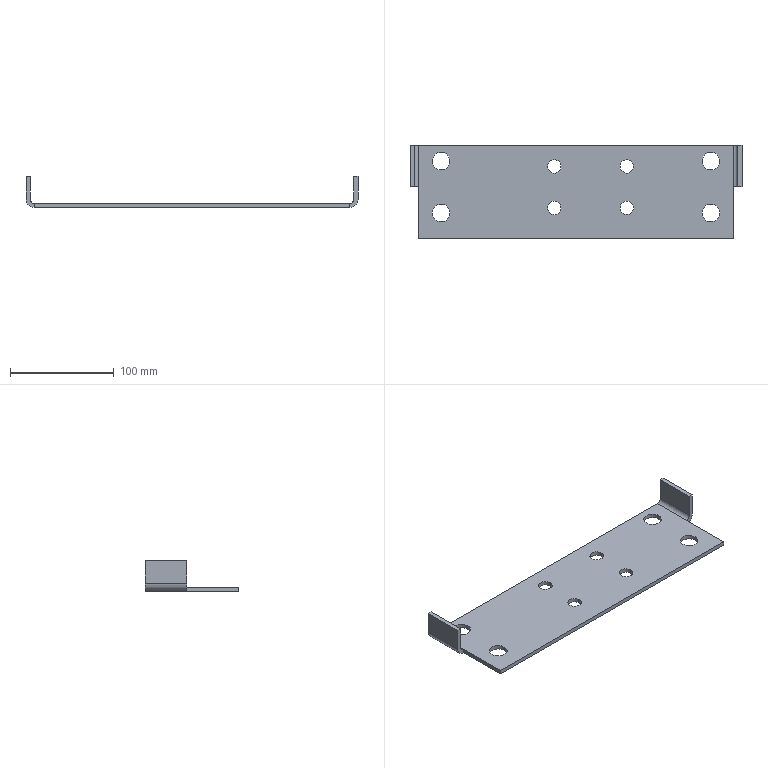Part | SolidWorks | features ICE 3, FlatPattern 1, SMBaseFlange 1, SheetMetal 1 | 1 solid | 38 faces | box 320 x 90.5 x 30 mm | volume 114349 mm3 | cylinder 20 | plane 18 | commonest cylinder face diameters 13 x8 17 x8 8 x2 16 x2
STEP:
#1=CARTESIAN_POINT('',(55.5,-15.25,4.));
#2=VERTEX_POINT('',#1);
#3=CARTESIAN_POINT('',(42.5,-15.25,4.));
#4=VERTEX_POINT('',#3);
#5=CARTESIAN_POINT('',(49.,-15.25,4.));
#6=DIRECTION('',(0.,0.,-1.));
#7=DIRECTION('',(-1.,0.,0.));
#8=AXIS2_PLACEMENT_3D('',#5,#6,#7);
#9=CIRCLE('',#8,6.5);
#10=EDGE_CURVE('',#2,#4,#9,.T.);
#11=ORIENTED_EDGE('',*,*,#10,.F.);
#12=CARTESIAN_POINT('',(55.5,-15.25,0.));
#13=VERTEX_POINT('',#12);
#14=CARTESIAN_POINT('',(55.5,-15.25,10.));
#15=DIRECTION('',(0.,0.,-1.));
#16=VECTOR('',#15,1000.);
#17=LINE('',#14,#16);
#18=EDGE_CURVE('',#2,#13,#17,.T.);
#19=ORIENTED_EDGE('',*,*,#18,.T.);
#20=CARTESIAN_POINT('',(42.5,-15.25,0.));
#21=VERTEX_POINT('',#20);
#22=CARTESIAN_POINT('',(49.,-15.25,0.));
#23=DIRECTION('',(0.,0.,-1.));
#24=DIRECTION('',(-1.,0.,0.));
#25=AXIS2_PLACEMENT_3D('',#22,#23,#24);
#26=CIRCLE('',#25,6.5);
#27=EDGE_CURVE('',#13,#21,#26,.T.);
#28=ORIENTED_EDGE('',*,*,#27,.T.);
#29=CARTESIAN_POINT('',(42.5,-15.25,10.));
#30=DIRECTION('',(0.,0.,-1.));
#31=VECTOR('',#30,1000.);
#32=LINE('',#29,#31);
#33=EDGE_CURVE('',#4,#21,#32,.T.);
#34=ORIENTED_EDGE('',*,*,#33,.F.);
#35=EDGE_LOOP('',(#11,#19,#28,#34));
#36=FACE_OUTER_BOUND('',#35,.T.);
#37=CARTESIAN_POINT('',(49.,-15.25,10.));
#38=DIRECTION('',(0.,0.,-1.));
#39=DIRECTION('',(-1.,0.,0.));
#40=AXIS2_PLACEMENT_3D('',#37,#38,#39);
#41=CYLINDRICAL_SURFACE('',#40,6.5);
#42=ADVANCED_FACE('',(#36),#41,.F.);
#43=CARTESIAN_POINT('',(-14.5,24.75,4.));
#44=VERTEX_POINT('',#43);
#45=CARTESIAN_POINT('',(-27.5,24.75,4.));
#46=VERTEX_POINT('',#45);
#47=CARTESIAN_POINT('',(-21.,24.75,4.));
#48=DIRECTION('',(0.,0.,-1.));
#49=DIRECTION('',(-1.,0.,0.));
#50=AXIS2_PLACEMENT_3D('',#47,#48,#49);
#51=CIRCLE('',#50,6.5);
#52=EDGE_CURVE('',#44,#46,#51,.T.);
#53=ORIENTED_EDGE('',*,*,#52,.F.);
#54=CARTESIAN_POINT('',(-14.5,24.75,0.));
#55=VERTEX_POINT('',#54);
#56=CARTESIAN_POINT('',(-14.5,24.75,10.));
#57=DIRECTION('',(0.,0.,-1.));
#58=VECTOR('',#57,1000.);
#59=LINE('',#56,#58);
#60=EDGE_CURVE('',#44,#55,#59,.T.);
#61=ORIENTED_EDGE('',*,*,#60,.T.);
#62=CARTESIAN_POINT('',(-27.5,24.75,0.));
#63=VERTEX_POINT('',#62);
#64=CARTESIAN_POINT('',(-21.,24.75,0.));
#65=DIRECTION('',(0.,0.,-1.));
#66=DIRECTION('',(-1.,0.,0.));
#67=AXIS2_PLACEMENT_3D('',#64,#65,#66);
#68=CIRCLE('',#67,6.5);
#69=EDGE_CURVE('',#55,#63,#68,.T.);
#70=ORIENTED_EDGE('',*,*,#69,.T.);
#71=CARTESIAN_POINT('',(-27.5,24.75,10.));
#72=DIRECTION('',(0.,0.,-1.));
#73=VECTOR('',#72,1000.);
#74=LINE('',#71,#73);
#75=EDGE_CURVE('',#46,#63,#74,.T.);
#76=ORIENTED_EDGE('',*,*,#75,.F.);
#77=EDGE_LOOP('',(#53,#61,#70,#76));
#78=FACE_OUTER_BOUND('',#77,.T.);
#79=CARTESIAN_POINT('',(-21.,24.75,10.));
#80=DIRECTION('',(0.,0.,-1.));
#81=DIRECTION('',(-1.,0.,0.));
#82=AXIS2_PLACEMENT_3D('',#79,#80,#81);
#83=CYLINDRICAL_SURFACE('',#82,6.5);
#84=ADVANCED_FACE('',(#78),#83,.F.);
#85=CARTESIAN_POINT('',(-14.5,-15.25,4.));
#86=VERTEX_POINT('',#85);
#87=CARTESIAN_POINT('',(-27.5,-15.25,4.));
#88=VERTEX_POINT('',#87);
#89=CARTESIAN_POINT('',(-21.,-15.25,4.));
#90=DIRECTION('',(0.,0.,-1.));
#91=DIRECTION('',(-1.,0.,0.));
#92=AXIS2_PLACEMENT_3D('',#89,#90,#91);
#93=CIRCLE('',#92,6.5);
#94=EDGE_CURVE('',#86,#88,#93,.T.);
#95=ORIENTED_EDGE('',*,*,#94,.F.);
#96=CARTESIAN_POINT('',(-14.5,-15.25,0.));
#97=VERTEX_POINT('',#96);
#98=CARTESIAN_POINT('',(-14.5,-15.25,10.));
#99=DIRECTION('',(0.,0.,-1.));
#100=VECTOR('',#99,1000.);
#101=LINE('',#98,#100);
#102=EDGE_CURVE('',#86,#97,#101,.T.);
#103=ORIENTED_EDGE('',*,*,#102,.T.);
#104=CARTESIAN_POINT('',(-27.5,-15.25,0.));
#105=VERTEX_POINT('',#104);
#106=CARTESIAN_POINT('',(-21.,-15.25,0.));
#107=DIRECTION('',(0.,0.,-1.));
#108=DIRECTION('',(-1.,0.,0.));
#109=AXIS2_PLACEMENT_3D('',#106,#107,#108);
#110=CIRCLE('',#109,6.5);
#111=EDGE_CURVE('',#97,#105,#110,.T.);
#112=ORIENTED_EDGE('',*,*,#111,.T.);
#113=CARTESIAN_POINT('',(-27.5,-15.25,10.));
#114=DIRECTION('',(0.,0.,-1.));
#115=VECTOR('',#114,1000.);
#116=LINE('',#113,#115);
#117=EDGE_CURVE('',#88,#105,#116,.T.);
#118=ORIENTED_EDGE('',*,*,#117,.F.);
#119=EDGE_LOOP('',(#95,#103,#112,#118));
#120=FACE_OUTER_BOUND('',#119,.T.);
#121=CARTESIAN_POINT('',(-21.,-15.25,10.));
#122=DIRECTION('',(0.,0.,-1.));
#123=DIRECTION('',(-1.,0.,0.));
#124=AXIS2_PLACEMENT_3D('',#121,#122,#123);
#125=CYLINDRICAL_SURFACE('',#124,6.5);
#126=ADVANCED_FACE('',(#120),#125,.F.);
#127=CARTESIAN_POINT('',(55.5,24.75,4.));
#128=VERTEX_POINT('',#127);
#129=CARTESIAN_POINT('',(42.5,24.75,4.));
#130=VERTEX_POINT('',#129);
#131=CARTESIAN_POINT('',(49.,24.75,4.));
#132=DIRECTION('',(0.,0.,-1.));
#133=DIRECTION('',(-1.,0.,0.));
#134=AXIS2_PLACEMENT_3D('',#131,#132,#133);
#135=CIRCLE('',#134,6.5);
#136=EDGE_CURVE('',#128,#130,#135,.T.);
#137=ORIENTED_EDGE('',*,*,#136,.F.);
#138=CARTESIAN_POINT('',(55.5,24.75,0.));
#139=VERTEX_POINT('',#138);
#140=CARTESIAN_POINT('',(55.5,24.75,10.));
#141=DIRECTION('',(0.,0.,-1.));
#142=VECTOR('',#141,1000.);
#143=LINE('',#140,#142);
#144=EDGE_CURVE('',#128,#139,#143,.T.);
#145=ORIENTED_EDGE('',*,*,#144,.T.);
#146=CARTESIAN_POINT('',(42.5,24.75,0.));
#147=VERTEX_POINT('',#146);
#148=CARTESIAN_POINT('',(49.,24.75,0.));
#149=DIRECTION('',(0.,0.,-1.));
#150=DIRECTION('',(-1.,0.,0.));
#151=AXIS2_PLACEMENT_3D('',#148,#149,#150);
#152=CIRCLE('',#151,6.5);
#153=EDGE_CURVE('',#139,#147,#152,.T.);
#154=ORIENTED_EDGE('',*,*,#153,.T.);
#155=CARTESIAN_POINT('',(42.5,24.75,10.));
#156=DIRECTION('',(0.,0.,-1.));
#157=VECTOR('',#156,1000.);
#158=LINE('',#155,#157);
#159=EDGE_CURVE('',#130,#147,#158,.T.);
#160=ORIENTED_EDGE('',*,*,#159,.F.);
#161=EDGE_LOOP('',(#137,#145,#154,#160));
#162=FACE_OUTER_BOUND('',#161,.T.);
#163=CARTESIAN_POINT('',(49.,24.75,10.));
#164=DIRECTION('',(0.,0.,-1.));
#165=DIRECTION('',(-1.,0.,0.));
#166=AXIS2_PLACEMENT_3D('',#163,#164,#165);
#167=CYLINDRICAL_SURFACE('',#166,6.5);
#168=ADVANCED_FACE('',(#162),#167,.F.);
#169=CARTESIAN_POINT('',(-121.5,-20.25,4.));
#170=VERTEX_POINT('',#169);
#171=CARTESIAN_POINT('',(-138.5,-20.25,4.));
#172=VERTEX_POINT('',#171);
#173=CARTESIAN_POINT('',(-130.,-20.25,4.));
#174=DIRECTION('',(0.,0.,-1.));
#175=DIRECTION('',(-1.,0.,0.));
#176=AXIS2_PLACEMENT_3D('',#173,#174,#175);
#177=CIRCLE('',#176,8.5);
#178=EDGE_CURVE('',#170,#172,#177,.T.);
#179=ORIENTED_EDGE('',*,*,#178,.F.);
#180=CARTESIAN_POINT('',(-121.5,-20.25,0.));
#181=VERTEX_POINT('',#180);
#182=CARTESIAN_POINT('',(-121.5,-20.25,10.));
#183=DIRECTION('',(0.,0.,-1.));
#184=VECTOR('',#183,1000.);
#185=LINE('',#182,#184);
#186=EDGE_CURVE('',#170,#181,#185,.T.);
#187=ORIENTED_EDGE('',*,*,#186,.T.);
#188=CARTESIAN_POINT('',(-138.5,-20.25,0.));
#189=VERTEX_POINT('',#188);
#190=CARTESIAN_POINT('',(-130.,-20.25,0.));
#191=DIRECTION('',(0.,0.,-1.));
#192=DIRECTION('',(-1.,0.,0.));
#193=AXIS2_PLACEMENT_3D('',#190,#191,#192);
#194=CIRCLE('',#193,8.5);
#195=EDGE_CURVE('',#181,#189,#194,.T.);
#196=ORIENTED_EDGE('',*,*,#195,.T.);
#197=CARTESIAN_POINT('',(-138.5,-20.25,10.));
#198=DIRECTION('',(0.,0.,-1.));
#199=VECTOR('',#198,1000.);
#200=LINE('',#197,#199);
#201=EDGE_CURVE('',#172,#189,#200,.T.);
#202=ORIENTED_EDGE('',*,*,#201,.F.);
#203=EDGE_LOOP('',(#179,#187,#196,#202));
#204=FACE_OUTER_BOUND('',#203,.T.);
#205=CARTESIAN_POINT('',(-130.,-20.25,10.));
#206=DIRECTION('',(0.,0.,-1.));
#207=DIRECTION('',(-1.,0.,0.));
#208=AXIS2_PLACEMENT_3D('',#205,#206,#207);
#209=CYLINDRICAL_SURFACE('',#208,8.5);
#210=ADVANCED_FACE('',(#204),#209,.F.);
#211=CARTESIAN_POINT('',(138.5,-20.25,4.));
#212=VERTEX_POINT('',#211);
#213=CARTESIAN_POINT('',(121.5,-20.25,4.));
#214=VERTEX_POINT('',#213);
#215=CARTESIAN_POINT('',(130.,-20.25,4.));
#216=DIRECTION('',(0.,0.,-1.));
#217=DIRECTION('',(-1.,0.,0.));
#218=AXIS2_PLACEMENT_3D('',#215,#216,#217);
#219=CIRCLE('',#218,8.5);
#220=EDGE_CURVE('',#212,#214,#219,.T.);
#221=ORIENTED_EDGE('',*,*,#220,.F.);
#222=CARTESIAN_POINT('',(138.5,-20.25,0.));
#223=VERTEX_POINT('',#222);
#224=CARTESIAN_POINT('',(138.5,-20.25,10.));
#225=DIRECTION('',(0.,0.,-1.));
#226=VECTOR('',#225,1000.);
#227=LINE('',#224,#226);
#228=EDGE_CURVE('',#212,#223,#227,.T.);
#229=ORIENTED_EDGE('',*,*,#228,.T.);
#230=CARTESIAN_POINT('',(121.5,-20.25,0.));
#231=VERTEX_POINT('',#230);
#232=CARTESIAN_POINT('',(130.,-20.25,0.));
#233=DIRECTION('',(0.,0.,-1.));
#234=DIRECTION('',(-1.,0.,0.));
#235=AXIS2_PLACEMENT_3D('',#232,#233,#234);
#236=CIRCLE('',#235,8.5);
#237=EDGE_CURVE('',#223,#231,#236,.T.);
#238=ORIENTED_EDGE('',*,*,#237,.T.);
#239=CARTESIAN_POINT('',(121.5,-20.25,10.));
#240=DIRECTION('',(0.,0.,-1.));
#241=VECTOR('',#240,1000.);
#242=LINE('',#239,#241);
#243=EDGE_CURVE('',#214,#231,#242,.T.);
#244=ORIENTED_EDGE('',*,*,#243,.F.);
#245=EDGE_LOOP('',(#221,#229,#238,#244));
#246=FACE_OUTER_BOUND('',#245,.T.);
#247=CARTESIAN_POINT('',(130.,-20.25,10.));
#248=DIRECTION('',(0.,0.,-1.));
#249=DIRECTION('',(-1.,0.,0.));
#250=AXIS2_PLACEMENT_3D('',#247,#248,#249);
#251=CYLINDRICAL_SURFACE('',#250,8.5);
#252=ADVANCED_FACE('',(#246),#251,.F.);
#253=CARTESIAN_POINT('',(138.5,29.75,4.));
#254=VERTEX_POINT('',#253);
#255=CARTESIAN_POINT('',(121.5,29.75,4.));
#256=VERTEX_POINT('',#255);
#257=CARTESIAN_POINT('',(130.,29.75,4.));
#258=DIRECTION('',(0.,0.,-1.));
#259=DIRECTION('',(-1.,0.,0.));
#260=AXIS2_PLACEMENT_3D('',#257,#258,#259);
#261=CIRCLE('',#260,8.5);
#262=EDGE_CURVE('',#254,#256,#261,.T.);
#263=ORIENTED_EDGE('',*,*,#262,.F.);
#264=CARTESIAN_POINT('',(138.5,29.75,0.));
#265=VERTEX_POINT('',#264);
#266=CARTESIAN_POINT('',(138.5,29.75,10.));
#267=DIRECTION('',(0.,0.,-1.));
#268=VECTOR('',#267,1000.);
#269=LINE('',#266,#268);
#270=EDGE_CURVE('',#254,#265,#269,.T.);
#271=ORIENTED_EDGE('',*,*,#270,.T.);
#272=CARTESIAN_POINT('',(121.5,29.75,0.));
#273=VERTEX_POINT('',#272);
#274=CARTESIAN_POINT('',(130.,29.75,0.));
#275=DIRECTION('',(0.,0.,-1.));
#276=DIRECTION('',(-1.,0.,0.));
#277=AXIS2_PLACEMENT_3D('',#274,#275,#276);
#278=CIRCLE('',#277,8.5);
#279=EDGE_CURVE('',#265,#273,#278,.T.);
#280=ORIENTED_EDGE('',*,*,#279,.T.);
#281=CARTESIAN_POINT('',(121.5,29.75,10.));
#282=DIRECTION('',(0.,0.,-1.));
#283=VECTOR('',#282,1000.);
#284=LINE('',#281,#283);
#285=EDGE_CURVE('',#256,#273,#284,.T.);
#286=ORIENTED_EDGE('',*,*,#285,.F.);
#287=EDGE_LOOP('',(#263,#271,#280,#286));
#288=FACE_OUTER_BOUND('',#287,.T.);
#289=CARTESIAN_POINT('',(130.,29.75,10.));
#290=DIRECTION('',(0.,0.,-1.));
#291=DIRECTION('',(-1.,0.,0.));
#292=AXIS2_PLACEMENT_3D('',#289,#290,#291);
#293=CYLINDRICAL_SURFACE('',#292,8.5);
#294=ADVANCED_FACE('',(#288),#293,.F.);
#295=CARTESIAN_POINT('',(-121.5,29.75,4.));
#296=VERTEX_POINT('',#295);
#297=CARTESIAN_POINT('',(-138.5,29.75,4.));
#298=VERTEX_POINT('',#297);
#299=CARTESIAN_POINT('',(-130.,29.75,4.));
#300=DIRECTION('',(0.,0.,-1.));
#301=DIRECTION('',(-1.,0.,0.));
#302=AXIS2_PLACEMENT_3D('',#299,#300,#301);
#303=CIRCLE('',#302,8.5);
#304=EDGE_CURVE('',#296,#298,#303,.T.);
#305=ORIENTED_EDGE('',*,*,#304,.F.);
#306=CARTESIAN_POINT('',(-121.5,29.75,0.));
#307=VERTEX_POINT('',#306);
#308=CARTESIAN_POINT('',(-121.5,29.75,10.));
#309=DIRECTION('',(0.,0.,-1.));
#310=VECTOR('',#309,1000.);
#311=LINE('',#308,#310);
#312=EDGE_CURVE('',#296,#307,#311,.T.);
#313=ORIENTED_EDGE('',*,*,#312,.T.);
#314=CARTESIAN_POINT('',(-138.5,29.75,0.));
#315=VERTEX_POINT('',#314);
#316=CARTESIAN_POINT('',(-130.,29.75,0.));
#317=DIRECTION('',(0.,0.,-1.));
#318=DIRECTION('',(-1.,0.,0.));
#319=AXIS2_PLACEMENT_3D('',#316,#317,#318);
#320=CIRCLE('',#319,8.5);
#321=EDGE_CURVE('',#307,#315,#320,.T.);
#322=ORIENTED_EDGE('',*,*,#321,.T.);
#323=CARTESIAN_POINT('',(-138.5,29.75,10.));
#324=DIRECTION('',(0.,0.,-1.));
#325=VECTOR('',#324,1000.);
#326=LINE('',#323,#325);
#327=EDGE_CURVE('',#298,#315,#326,.T.);
#328=ORIENTED_EDGE('',*,*,#327,.F.);
#329=EDGE_LOOP('',(#305,#313,#322,#328));
#330=FACE_OUTER_BOUND('',#329,.T.);
#331=CARTESIAN_POINT('',(-130.,29.75,10.));
#332=DIRECTION('',(0.,0.,-1.));
#333=DIRECTION('',(-1.,0.,0.));
#334=AXIS2_PLACEMENT_3D('',#331,#332,#333);
#335=CYLINDRICAL_SURFACE('',#334,8.5);
#336=ADVANCED_FACE('',(#330),#335,.F.);
#337=CARTESIAN_POINT('',(-152.,45.25,0.));
#338=VERTEX_POINT('',#337);
#339=CARTESIAN_POINT('',(-152.,45.25,4.));
#340=VERTEX_POINT('',#339);
#341=CARTESIAN_POINT('',(-152.,45.25,0.));
#342=DIRECTION('',(0.,0.,1.));
#343=VECTOR('',#342,1000.);
#344=LINE('',#341,#343);
#345=EDGE_CURVE('',#338,#340,#344,.T.);
#346=ORIENTED_EDGE('',*,*,#345,.F.);
#347=CARTESIAN_POINT('',(-160.,45.25,8.));
#348=VERTEX_POINT('',#347);
#349=CARTESIAN_POINT('',(-152.,45.25,8.));
#350=DIRECTION('',(0.,-1.,0.));
#351=DIRECTION('',(0.,0.,1.));
#352=AXIS2_PLACEMENT_3D('',#349,#350,#351);
#353=CIRCLE('',#352,8.);
#354=EDGE_CURVE('',#348,#338,#353,.T.);
#355=ORIENTED_EDGE('',*,*,#354,.F.);
#356=CARTESIAN_POINT('',(-156.,45.25,8.));
#357=VERTEX_POINT('',#356);
#358=CARTESIAN_POINT('',(-156.,45.25,8.));
#359=DIRECTION('',(-1.,0.,0.));
#360=VECTOR('',#359,1000.);
#361=LINE('',#358,#360);
#362=EDGE_CURVE('',#357,#348,#361,.T.);
#363=ORIENTED_EDGE('',*,*,#362,.F.);
#364=CARTESIAN_POINT('',(-152.,45.25,8.));
#365=DIRECTION('',(0.,-1.,0.));
#366=DIRECTION('',(1.,0.,0.));
#367=AXIS2_PLACEMENT_3D('',#364,#365,#366);
#368=CIRCLE('',#367,4.);
#369=EDGE_CURVE('',#357,#340,#368,.T.);
#370=ORIENTED_EDGE('',*,*,#369,.T.);
#371=EDGE_LOOP('',(#346,#355,#363,#370));
#372=FACE_OUTER_BOUND('',#371,.T.);
#373=CARTESIAN_POINT('',(-152.,45.25,0.));
#374=DIRECTION('',(0.,1.,0.));
#375=DIRECTION('',(0.,0.,1.));
#376=AXIS2_PLACEMENT_3D('',#373,#374,#375);
#377=PLANE('',#376);
#378=ADVANCED_FACE('',(#372),#377,.T.);
#379=CARTESIAN_POINT('',(152.,45.25,0.));
#380=VERTEX_POINT('',#379);
#381=CARTESIAN_POINT('',(-160.,45.25,0.));
#382=DIRECTION('',(1.,0.,0.));
#383=VECTOR('',#382,1000.);
#384=LINE('',#381,#383);
#385=EDGE_CURVE('',#338,#380,#384,.T.);
#386=ORIENTED_EDGE('',*,*,#385,.F.);
#387=ORIENTED_EDGE('',*,*,#345,.T.);
#388=CARTESIAN_POINT('',(152.,45.25,4.));
#389=VERTEX_POINT('',#388);
#390=CARTESIAN_POINT('',(-160.,45.25,4.));
#391=DIRECTION('',(1.,0.,0.));
#392=VECTOR('',#391,1000.);
#393=LINE('',#390,#392);
#394=EDGE_CURVE('',#340,#389,#393,.T.);
#395=ORIENTED_EDGE('',*,*,#394,.T.);
#396=CARTESIAN_POINT('',(152.,45.25,4.));
#397=DIRECTION('',(0.,0.,-1.));
#398=VECTOR('',#397,1000.);
#399=LINE('',#396,#398);
#400=EDGE_CURVE('',#389,#380,#399,.T.);
#401=ORIENTED_EDGE('',*,*,#400,.T.);
#402=EDGE_LOOP('',(#386,#387,#395,#401));
#403=FACE_OUTER_BOUND('',#402,.T.);
#404=CARTESIAN_POINT('',(-156.,45.25,8.));
#405=DIRECTION('',(0.,1.,0.));
#406=DIRECTION('',(0.,0.,1.));
#407=AXIS2_PLACEMENT_3D('',#404,#405,#406);
#408=PLANE('',#407);
#409=ADVANCED_FACE('',(#403),#408,.T.);
#410=CARTESIAN_POINT('',(160.,45.25,8.));
#411=VERTEX_POINT('',#410);
#412=CARTESIAN_POINT('',(156.,45.25,8.));
#413=VERTEX_POINT('',#412);
#414=CARTESIAN_POINT('',(160.,45.25,8.));
#415=DIRECTION('',(-1.,0.,0.));
#416=VECTOR('',#415,1000.);
#417=LINE('',#414,#416);
#418=EDGE_CURVE('',#411,#413,#417,.T.);
#419=ORIENTED_EDGE('',*,*,#418,.F.);
#420=CARTESIAN_POINT('',(152.,45.25,8.));
#421=DIRECTION('',(0.,-1.,0.));
#422=DIRECTION('',(0.,0.,1.));
#423=AXIS2_PLACEMENT_3D('',#420,#421,#422);
#424=CIRCLE('',#423,8.);
#425=EDGE_CURVE('',#380,#411,#424,.T.);
#426=ORIENTED_EDGE('',*,*,#425,.F.);
#427=ORIENTED_EDGE('',*,*,#400,.F.);
#428=CARTESIAN_POINT('',(152.,45.25,8.));
#429=DIRECTION('',(0.,-1.,0.));
#430=DIRECTION('',(1.,0.,0.));
#431=AXIS2_PLACEMENT_3D('',#428,#429,#430);
#432=CIRCLE('',#431,4.);
#433=EDGE_CURVE('',#389,#413,#432,.T.);
#434=ORIENTED_EDGE('',*,*,#433,.T.);
#435=EDGE_LOOP('',(#419,#426,#427,#434));
#436=FACE_OUTER_BOUND('',#435,.T.);
#437=CARTESIAN_POINT('',(160.,45.25,8.));
#438=DIRECTION('',(0.,1.,0.));
#439=DIRECTION('',(0.,0.,1.));
#440=AXIS2_PLACEMENT_3D('',#437,#438,#439);
#441=PLANE('',#440);
#442=ADVANCED_FACE('',(#436),#441,.T.);
#443=CARTESIAN_POINT('',(160.,45.25,30.));
#444=VERTEX_POINT('',#443);
#445=CARTESIAN_POINT('',(160.,45.25,0.));
#446=DIRECTION('',(0.,0.,1.));
#447=VECTOR('',#446,1000.);
#448=LINE('',#445,#447);
#449=EDGE_CURVE('',#411,#444,#448,.T.);
#450=ORIENTED_EDGE('',*,*,#449,.F.);
#451=ORIENTED_EDGE('',*,*,#418,.T.);
#452=CARTESIAN_POINT('',(156.,45.25,30.));
#453=VERTEX_POINT('',#452);
#454=CARTESIAN_POINT('',(156.,45.25,0.));
#455=DIRECTION('',(0.,0.,1.));
#456=VECTOR('',#455,1000.);
#457=LINE('',#454,#456);
#458=EDGE_CURVE('',#413,#453,#457,.T.);
#459=ORIENTED_EDGE('',*,*,#458,.T.);
#460=CARTESIAN_POINT('',(160.,45.25,30.));
#461=DIRECTION('',(-1.,0.,0.));
#462=VECTOR('',#461,1000.);
#463=LINE('',#460,#462);
#464=EDGE_CURVE('',#444,#453,#463,.T.);
#465=ORIENTED_EDGE('',*,*,#464,.F.);
#466=EDGE_LOOP('',(#450,#451,#459,#465));
#467=FACE_OUTER_BOUND('',#466,.T.);
#468=CARTESIAN_POINT('',(152.,45.25,4.));
#469=DIRECTION('',(0.,1.,0.));
#470=DIRECTION('',(0.,0.,1.));
#471=AXIS2_PLACEMENT_3D('',#468,#469,#470);
#472=PLANE('',#471);
#473=ADVANCED_FACE('',(#467),#472,.T.);
#474=CARTESIAN_POINT('',(-152.,-45.25,0.));
#475=VERTEX_POINT('',#474);
#476=CARTESIAN_POINT('',(152.,-45.25,0.));
#477=VERTEX_POINT('',#476);
#478=CARTESIAN_POINT('',(-160.,-45.25,0.));
#479=DIRECTION('',(1.,0.,0.));
#480=VECTOR('',#479,1000.);
#481=LINE('',#478,#480);
#482=EDGE_CURVE('',#475,#477,#481,.T.);
#483=ORIENTED_EDGE('',*,*,#482,.T.);
#484=CARTESIAN_POINT('',(152.,-45.25,4.));
#485=VERTEX_POINT('',#484);
#486=CARTESIAN_POINT('',(152.,-45.25,0.));
#487=DIRECTION('',(0.,0.,1.));
#488=VECTOR('',#487,1000.);
#489=LINE('',#486,#488);
#490=EDGE_CURVE('',#477,#485,#489,.T.);
#491=ORIENTED_EDGE('',*,*,#490,.T.);
#492=CARTESIAN_POINT('',(-152.,-45.25,4.));
#493=VERTEX_POINT('',#492);
#494=CARTESIAN_POINT('',(-160.,-45.25,4.));
#495=DIRECTION('',(1.,0.,0.));
#496=VECTOR('',#495,1000.);
#497=LINE('',#494,#496);
#498=EDGE_CURVE('',#493,#485,#497,.T.);
#499=ORIENTED_EDGE('',*,*,#498,.F.);
#500=CARTESIAN_POINT('',(-152.,-45.25,4.));
#501=DIRECTION('',(0.,0.,-1.));
#502=VECTOR('',#501,1000.);
#503=LINE('',#500,#502);
#504=EDGE_CURVE('',#493,#475,#503,.T.);
#505=ORIENTED_EDGE('',*,*,#504,.T.);
#506=EDGE_LOOP('',(#483,#491,#499,#505));
#507=FACE_OUTER_BOUND('',#506,.T.);
#508=CARTESIAN_POINT('',(156.,-45.25,8.));
#509=DIRECTION('',(0.,-1.,0.));
#510=DIRECTION('',(0.,0.,-1.));
#511=AXIS2_PLACEMENT_3D('',#508,#509,#510);
#512=PLANE('',#511);
#513=ADVANCED_FACE('',(#507),#512,.T.);
#514=CARTESIAN_POINT('',(156.,5.25,8.));
#515=VERTEX_POINT('',#514);
#516=CARTESIAN_POINT('',(156.,45.25,8.));
#517=DIRECTION('',(0.,-1.,0.));
#518=VECTOR('',#517,1000.);
#519=LINE('',#516,#518);
#520=EDGE_CURVE('',#413,#515,#519,.T.);
#521=ORIENTED_EDGE('',*,*,#520,.T.);
#522=CARTESIAN_POINT('',(156.,5.25,30.));
#523=VERTEX_POINT('',#522);
#524=CARTESIAN_POINT('',(156.,5.25,0.));
#525=DIRECTION('',(0.,0.,1.));
#526=VECTOR('',#525,1000.);
#527=LINE('',#524,#526);
#528=EDGE_CURVE('',#515,#523,#527,.T.);
#529=ORIENTED_EDGE('',*,*,#528,.T.);
#530=CARTESIAN_POINT('',(156.,45.25,30.));
#531=DIRECTION('',(0.,-1.,0.));
#532=VECTOR('',#531,1000.);
#533=LINE('',#530,#532);
#534=EDGE_CURVE('',#453,#523,#533,.T.);
#535=ORIENTED_EDGE('',*,*,#534,.F.);
#536=ORIENTED_EDGE('',*,*,#458,.F.);
#537=EDGE_LOOP('',(#521,#529,#535,#536));
#538=FACE_OUTER_BOUND('',#537,.T.);
#539=CARTESIAN_POINT('',(156.,45.25,0.));
#540=DIRECTION('',(1.,0.,0.));
#541=DIRECTION('',(0.,0.,-1.));
#542=AXIS2_PLACEMENT_3D('',#539,#540,#541);
#543=PLANE('',#542);
#544=ADVANCED_FACE('',(#538),#543,.F.);
#545=CARTESIAN_POINT('',(160.,5.25,30.));
#546=VERTEX_POINT('',#545);
#547=CARTESIAN_POINT('',(160.,5.25,30.));
#548=DIRECTION('',(-1.,0.,0.));
#549=VECTOR('',#548,1000.);
#550=LINE('',#547,#549);
#551=EDGE_CURVE('',#546,#523,#550,.T.);
#552=ORIENTED_EDGE('',*,*,#551,.F.);
#553=CARTESIAN_POINT('',(160.,45.25,30.));
#554=DIRECTION('',(0.,-1.,0.));
#555=VECTOR('',#554,1000.);
#556=LINE('',#553,#555);
#557=EDGE_CURVE('',#444,#546,#556,.T.);
#558=ORIENTED_EDGE('',*,*,#557,.F.);
#559=ORIENTED_EDGE('',*,*,#464,.T.);
#560=ORIENTED_EDGE('',*,*,#534,.T.);
#561=EDGE_LOOP('',(#552,#558,#559,#560));
#562=FACE_OUTER_BOUND('',#561,.T.);
#563=CARTESIAN_POINT('',(160.,45.25,30.));
#564=DIRECTION('',(0.,0.,1.));
#565=DIRECTION('',(1.,0.,0.));
#566=AXIS2_PLACEMENT_3D('',#563,#564,#565);
#567=PLANE('',#566);
#568=ADVANCED_FACE('',(#562),#567,.T.);
#569=CARTESIAN_POINT('',(160.,5.25,8.));
#570=VERTEX_POINT('',#569);
#571=CARTESIAN_POINT('',(160.,5.25,0.));
#572=DIRECTION('',(0.,0.,1.));
#573=VECTOR('',#572,1000.);
#574=LINE('',#571,#573);
#575=EDGE_CURVE('',#570,#546,#574,.T.);
#576=ORIENTED_EDGE('',*,*,#575,.F.);
#577=CARTESIAN_POINT('',(160.,45.25,8.));
#578=DIRECTION('',(0.,-1.,0.));
#579=VECTOR('',#578,1000.);
#580=LINE('',#577,#579);
#581=EDGE_CURVE('',#411,#570,#580,.T.);
#582=ORIENTED_EDGE('',*,*,#581,.F.);
#583=ORIENTED_EDGE('',*,*,#449,.T.);
#584=ORIENTED_EDGE('',*,*,#557,.T.);
#585=EDGE_LOOP('',(#576,#582,#583,#584));
#586=FACE_OUTER_BOUND('',#585,.T.);
#587=CARTESIAN_POINT('',(160.,45.25,0.));
#588=DIRECTION('',(1.,0.,0.));
#589=DIRECTION('',(0.,0.,-1.));
#590=AXIS2_PLACEMENT_3D('',#587,#588,#589);
#591=PLANE('',#590);
#592=ADVANCED_FACE('',(#586),#591,.T.);
#593=CARTESIAN_POINT('',(152.,5.25,0.));
#594=VERTEX_POINT('',#593);
#595=CARTESIAN_POINT('',(152.,5.25,8.));
#596=DIRECTION('',(0.,-1.,0.));
#597=DIRECTION('',(0.,0.,1.));
#598=AXIS2_PLACEMENT_3D('',#595,#596,#597);
#599=CIRCLE('',#598,8.);
#600=EDGE_CURVE('',#594,#570,#599,.T.);
#601=ORIENTED_EDGE('',*,*,#600,.F.);
#602=CARTESIAN_POINT('',(152.,45.25,0.));
#603=DIRECTION('',(0.,-1.,0.));
#604=VECTOR('',#603,1000.);
#605=LINE('',#602,#604);
#606=EDGE_CURVE('',#380,#594,#605,.T.);
#607=ORIENTED_EDGE('',*,*,#606,.F.);
#608=ORIENTED_EDGE('',*,*,#425,.T.);
#609=ORIENTED_EDGE('',*,*,#581,.T.);
#610=EDGE_LOOP('',(#601,#607,#608,#609));
#611=FACE_OUTER_BOUND('',#610,.T.);
#612=CARTESIAN_POINT('',(152.,45.25,8.));
#613=DIRECTION('',(0.,-1.,0.));
#614=DIRECTION('',(0.,0.,-1.));
#615=AXIS2_PLACEMENT_3D('',#612,#613,#614);
#616=CYLINDRICAL_SURFACE('',#615,8.);
#617=ADVANCED_FACE('',(#611),#616,.T.);
#618=CARTESIAN_POINT('',(49.,-15.25,0.));
#619=DIRECTION('',(0.,0.,-1.));
#620=DIRECTION('',(-1.,0.,0.));
#621=AXIS2_PLACEMENT_3D('',#618,#619,#620);
#622=CIRCLE('',#621,6.5);
#623=EDGE_CURVE('',#21,#13,#622,.T.);
#624=ORIENTED_EDGE('',*,*,#623,.F.);
#625=ORIENTED_EDGE('',*,*,#27,.F.);
#626=EDGE_LOOP('',(#624,#625));
#627=FACE_BOUND('',#626,.T.);
#628=CARTESIAN_POINT('',(-21.,24.75,0.));
#629=DIRECTION('',(0.,0.,-1.));
#630=DIRECTION('',(-1.,0.,0.));
#631=AXIS2_PLACEMENT_3D('',#628,#629,#630);
#632=CIRCLE('',#631,6.5);
#633=EDGE_CURVE('',#63,#55,#632,.T.);
#634=ORIENTED_EDGE('',*,*,#633,.F.);
#635=ORIENTED_EDGE('',*,*,#69,.F.);
#636=EDGE_LOOP('',(#634,#635));
#637=FACE_BOUND('',#636,.T.);
#638=CARTESIAN_POINT('',(-21.,-15.25,0.));
#639=DIRECTION('',(0.,0.,-1.));
#640=DIRECTION('',(-1.,0.,0.));
#641=AXIS2_PLACEMENT_3D('',#638,#639,#640);
#642=CIRCLE('',#641,6.5);
#643=EDGE_CURVE('',#105,#97,#642,.T.);
#644=ORIENTED_EDGE('',*,*,#643,.F.);
#645=ORIENTED_EDGE('',*,*,#111,.F.);
#646=EDGE_LOOP('',(#644,#645));
#647=FACE_BOUND('',#646,.T.);
#648=CARTESIAN_POINT('',(49.,24.75,0.));
#649=DIRECTION('',(0.,0.,-1.));
#650=DIRECTION('',(-1.,0.,0.));
#651=AXIS2_PLACEMENT_3D('',#648,#649,#650);
#652=CIRCLE('',#651,6.5);
#653=EDGE_CURVE('',#147,#139,#652,.T.);
#654=ORIENTED_EDGE('',*,*,#653,.F.);
#655=ORIENTED_EDGE('',*,*,#153,.F.);
#656=EDGE_LOOP('',(#654,#655));
#657=FACE_BOUND('',#656,.T.);
#658=CARTESIAN_POINT('',(-130.,-20.25,0.));
#659=DIRECTION('',(0.,0.,-1.));
#660=DIRECTION('',(-1.,0.,0.));
#661=AXIS2_PLACEMENT_3D('',#658,#659,#660);
#662=CIRCLE('',#661,8.5);
#663=EDGE_CURVE('',#189,#181,#662,.T.);
#664=ORIENTED_EDGE('',*,*,#663,.F.);
#665=ORIENTED_EDGE('',*,*,#195,.F.);
#666=EDGE_LOOP('',(#664,#665));
#667=FACE_BOUND('',#666,.T.);
#668=CARTESIAN_POINT('',(130.,-20.25,0.));
#669=DIRECTION('',(0.,0.,-1.));
#670=DIRECTION('',(-1.,0.,0.));
#671=AXIS2_PLACEMENT_3D('',#668,#669,#670);
#672=CIRCLE('',#671,8.5);
#673=EDGE_CURVE('',#231,#223,#672,.T.);
#674=ORIENTED_EDGE('',*,*,#673,.F.);
#675=ORIENTED_EDGE('',*,*,#237,.F.);
#676=EDGE_LOOP('',(#674,#675));
#677=FACE_BOUND('',#676,.T.);
#678=CARTESIAN_POINT('',(130.,29.75,0.));
#679=DIRECTION('',(0.,0.,-1.));
#680=DIRECTION('',(-1.,0.,0.));
#681=AXIS2_PLACEMENT_3D('',#678,#679,#680);
#682=CIRCLE('',#681,8.5);
#683=EDGE_CURVE('',#273,#265,#682,.T.);
#684=ORIENTED_EDGE('',*,*,#683,.F.);
#685=ORIENTED_EDGE('',*,*,#279,.F.);
#686=EDGE_LOOP('',(#684,#685));
#687=FACE_BOUND('',#686,.T.);
#688=CARTESIAN_POINT('',(-130.,29.75,0.));
#689=DIRECTION('',(0.,0.,-1.));
#690=DIRECTION('',(-1.,0.,0.));
#691=AXIS2_PLACEMENT_3D('',#688,#689,#690);
#692=CIRCLE('',#691,8.5);
#693=EDGE_CURVE('',#315,#307,#692,.T.);
#694=ORIENTED_EDGE('',*,*,#693,.F.);
#695=ORIENTED_EDGE('',*,*,#321,.F.);
#696=EDGE_LOOP('',(#694,#695));
#697=FACE_BOUND('',#696,.T.);
#698=ORIENTED_EDGE('',*,*,#482,.F.);
#699=CARTESIAN_POINT('',(-152.,5.25,0.));
#700=VERTEX_POINT('',#699);
#701=CARTESIAN_POINT('',(-152.,-45.25,0.));
#702=DIRECTION('',(0.,1.,0.));
#703=VECTOR('',#702,1000.);
#704=LINE('',#701,#703);
#705=EDGE_CURVE('',#475,#700,#704,.T.);
#706=ORIENTED_EDGE('',*,*,#705,.T.);
#707=CARTESIAN_POINT('',(-152.,45.25,0.));
#708=DIRECTION('',(0.,-1.,0.));
#709=VECTOR('',#708,1000.);
#710=LINE('',#707,#709);
#711=EDGE_CURVE('',#338,#700,#710,.T.);
#712=ORIENTED_EDGE('',*,*,#711,.F.);
#713=ORIENTED_EDGE('',*,*,#385,.T.);
#714=ORIENTED_EDGE('',*,*,#606,.T.);
#715=CARTESIAN_POINT('',(152.,-45.25,0.));
#716=DIRECTION('',(0.,-1.,0.));
#717=VECTOR('',#716,1000.);
#718=LINE('',#715,#717);
#719=EDGE_CURVE('',#594,#477,#718,.T.);
#720=ORIENTED_EDGE('',*,*,#719,.T.);
#721=EDGE_LOOP('',(#698,#706,#712,#713,#714,#720));
#722=FACE_OUTER_BOUND('',#721,.T.);
#723=CARTESIAN_POINT('',(-160.,45.25,0.));
#724=DIRECTION('',(0.,0.,-1.));
#725=DIRECTION('',(-1.,0.,0.));
#726=AXIS2_PLACEMENT_3D('',#723,#724,#725);
#727=PLANE('',#726);
#728=ADVANCED_FACE('',(#627,#637,#647,#657,#667,#677,#687,#697,#722),#727,.T.);
#729=CARTESIAN_POINT('',(-160.,5.25,8.));
#730=VERTEX_POINT('',#729);
#731=CARTESIAN_POINT('',(-152.,5.25,8.));
#732=DIRECTION('',(0.,-1.,0.));
#733=DIRECTION('',(0.,0.,1.));
#734=AXIS2_PLACEMENT_3D('',#731,#732,#733);
#735=CIRCLE('',#734,8.);
#736=EDGE_CURVE('',#730,#700,#735,.T.);
#737=ORIENTED_EDGE('',*,*,#736,.F.);
#738=CARTESIAN_POINT('',(-160.,45.25,8.));
#739=DIRECTION('',(0.,-1.,0.));
#740=VECTOR('',#739,1000.);
#741=LINE('',#738,#740);
#742=EDGE_CURVE('',#348,#730,#741,.T.);
#743=ORIENTED_EDGE('',*,*,#742,.F.);
#744=ORIENTED_EDGE('',*,*,#354,.T.);
#745=ORIENTED_EDGE('',*,*,#711,.T.);
#746=EDGE_LOOP('',(#737,#743,#744,#745));
#747=FACE_OUTER_BOUND('',#746,.T.);
#748=CARTESIAN_POINT('',(-152.,45.25,8.));
#749=DIRECTION('',(0.,-1.,0.));
#750=DIRECTION('',(0.,0.,-1.));
#751=AXIS2_PLACEMENT_3D('',#748,#749,#750);
#752=CYLINDRICAL_SURFACE('',#751,8.);
#753=ADVANCED_FACE('',(#747),#752,.T.);
#754=CARTESIAN_POINT('',(-160.,5.25,30.));
#755=VERTEX_POINT('',#754);
#756=CARTESIAN_POINT('',(-160.,5.25,0.));
#757=DIRECTION('',(0.,0.,1.));
#758=VECTOR('',#757,1000.);
#759=LINE('',#756,#758);
#760=EDGE_CURVE('',#730,#755,#759,.T.);
#761=ORIENTED_EDGE('',*,*,#760,.T.);
#762=CARTESIAN_POINT('',(-160.,45.25,30.));
#763=VERTEX_POINT('',#762);
#764=CARTESIAN_POINT('',(-160.,45.25,30.));
#765=DIRECTION('',(0.,-1.,0.));
#766=VECTOR('',#765,1000.);
#767=LINE('',#764,#766);
#768=EDGE_CURVE('',#763,#755,#767,.T.);
#769=ORIENTED_EDGE('',*,*,#768,.F.);
#770=CARTESIAN_POINT('',(-160.,45.25,30.));
#771=DIRECTION('',(0.,0.,-1.));
#772=VECTOR('',#771,1000.);
#773=LINE('',#770,#772);
#774=EDGE_CURVE('',#763,#348,#773,.T.);
#775=ORIENTED_EDGE('',*,*,#774,.T.);
#776=ORIENTED_EDGE('',*,*,#742,.T.);
#777=EDGE_LOOP('',(#761,#769,#775,#776));
#778=FACE_OUTER_BOUND('',#777,.T.);
#779=CARTESIAN_POINT('',(-160.,45.25,30.));
#780=DIRECTION('',(-1.,0.,0.));
#781=DIRECTION('',(0.,0.,1.));
#782=AXIS2_PLACEMENT_3D('',#779,#780,#781);
#783=PLANE('',#782);
#784=ADVANCED_FACE('',(#778),#783,.T.);
#785=CARTESIAN_POINT('',(-156.,5.25,30.));
#786=VERTEX_POINT('',#785);
#787=CARTESIAN_POINT('',(-160.,5.25,30.));
#788=DIRECTION('',(-1.,0.,0.));
#789=VECTOR('',#788,1000.);
#790=LINE('',#787,#789);
#791=EDGE_CURVE('',#786,#755,#790,.T.);
#792=ORIENTED_EDGE('',*,*,#791,.F.);
#793=CARTESIAN_POINT('',(-156.,45.25,30.));
#794=VERTEX_POINT('',#793);
#795=CARTESIAN_POINT('',(-156.,45.25,30.));
#796=DIRECTION('',(0.,-1.,0.));
#797=VECTOR('',#796,1000.);
#798=LINE('',#795,#797);
#799=EDGE_CURVE('',#794,#786,#798,.T.);
#800=ORIENTED_EDGE('',*,*,#799,.F.);
#801=CARTESIAN_POINT('',(-156.,45.25,30.));
#802=DIRECTION('',(-1.,0.,0.));
#803=VECTOR('',#802,1000.);
#804=LINE('',#801,#803);
#805=EDGE_CURVE('',#794,#763,#804,.T.);
#806=ORIENTED_EDGE('',*,*,#805,.T.);
#807=ORIENTED_EDGE('',*,*,#768,.T.);
#808=EDGE_LOOP('',(#792,#800,#806,#807));
#809=FACE_OUTER_BOUND('',#808,.T.);
#810=CARTESIAN_POINT('',(-156.,45.25,30.));
#811=DIRECTION('',(0.,0.,1.));
#812=DIRECTION('',(1.,0.,0.));
#813=AXIS2_PLACEMENT_3D('',#810,#811,#812);
#814=PLANE('',#813);
#815=ADVANCED_FACE('',(#809),#814,.T.);
#816=ORIENTED_EDGE('',*,*,#799,.T.);
#817=CARTESIAN_POINT('',(-156.,5.25,8.));
#818=VERTEX_POINT('',#817);
#819=CARTESIAN_POINT('',(-156.,5.25,30.));
#820=DIRECTION('',(0.,0.,-1.));
#821=VECTOR('',#820,1000.);
#822=LINE('',#819,#821);
#823=EDGE_CURVE('',#786,#818,#822,.T.);
#824=ORIENTED_EDGE('',*,*,#823,.T.);
#825=CARTESIAN_POINT('',(-156.,45.25,8.));
#826=DIRECTION('',(0.,-1.,0.));
#827=VECTOR('',#826,1000.);
#828=LINE('',#825,#827);
#829=EDGE_CURVE('',#357,#818,#828,.T.);
#830=ORIENTED_EDGE('',*,*,#829,.F.);
#831=CARTESIAN_POINT('',(-156.,45.25,30.));
#832=DIRECTION('',(0.,0.,-1.));
#833=VECTOR('',#832,1000.);
#834=LINE('',#831,#833);
#835=EDGE_CURVE('',#794,#357,#834,.T.);
#836=ORIENTED_EDGE('',*,*,#835,.F.);
#837=EDGE_LOOP('',(#816,#824,#830,#836));
#838=FACE_OUTER_BOUND('',#837,.T.);
#839=CARTESIAN_POINT('',(-156.,45.25,30.));
#840=DIRECTION('',(-1.,0.,0.));
#841=DIRECTION('',(0.,0.,1.));
#842=AXIS2_PLACEMENT_3D('',#839,#840,#841);
#843=PLANE('',#842);
#844=ADVANCED_FACE('',(#838),#843,.F.);
#845=ORIENTED_EDGE('',*,*,#829,.T.);
#846=CARTESIAN_POINT('',(-152.,5.25,4.));
#847=VERTEX_POINT('',#846);
#848=CARTESIAN_POINT('',(-152.,5.25,8.));
#849=DIRECTION('',(0.,-1.,0.));
#850=DIRECTION('',(0.,0.,1.));
#851=AXIS2_PLACEMENT_3D('',#848,#849,#850);
#852=CIRCLE('',#851,4.);
#853=EDGE_CURVE('',#818,#847,#852,.T.);
#854=ORIENTED_EDGE('',*,*,#853,.T.);
#855=CARTESIAN_POINT('',(-152.,45.25,4.));
#856=DIRECTION('',(0.,-1.,0.));
#857=VECTOR('',#856,1000.);
#858=LINE('',#855,#857);
#859=EDGE_CURVE('',#340,#847,#858,.T.);
#860=ORIENTED_EDGE('',*,*,#859,.F.);
#861=ORIENTED_EDGE('',*,*,#369,.F.);
#862=EDGE_LOOP('',(#845,#854,#860,#861));
#863=FACE_OUTER_BOUND('',#862,.T.);
#864=CARTESIAN_POINT('',(-152.,45.25,8.));
#865=DIRECTION('',(0.,-1.,0.));
#866=DIRECTION('',(0.,0.,-1.));
#867=AXIS2_PLACEMENT_3D('',#864,#865,#866);
#868=CYLINDRICAL_SURFACE('',#867,4.);
#869=ADVANCED_FACE('',(#863),#868,.F.);
#870=CARTESIAN_POINT('',(49.,-15.25,4.));
#871=DIRECTION('',(0.,0.,-1.));
#872=DIRECTION('',(-1.,0.,0.));
#873=AXIS2_PLACEMENT_3D('',#870,#871,#872);
#874=CIRCLE('',#873,6.5);
#875=EDGE_CURVE('',#4,#2,#874,.T.);
#876=ORIENTED_EDGE('',*,*,#875,.T.);
#877=ORIENTED_EDGE('',*,*,#10,.T.);
#878=EDGE_LOOP('',(#876,#877));
#879=FACE_BOUND('',#878,.T.);
#880=CARTESIAN_POINT('',(-21.,24.75,4.));
#881=DIRECTION('',(0.,0.,-1.));
#882=DIRECTION('',(-1.,0.,0.));
#883=AXIS2_PLACEMENT_3D('',#880,#881,#882);
#884=CIRCLE('',#883,6.5);
#885=EDGE_CURVE('',#46,#44,#884,.T.);
#886=ORIENTED_EDGE('',*,*,#885,.T.);
#887=ORIENTED_EDGE('',*,*,#52,.T.);
#888=EDGE_LOOP('',(#886,#887));
#889=FACE_BOUND('',#888,.T.);
#890=CARTESIAN_POINT('',(-21.,-15.25,4.));
#891=DIRECTION('',(0.,0.,-1.));
#892=DIRECTION('',(-1.,0.,0.));
#893=AXIS2_PLACEMENT_3D('',#890,#891,#892);
#894=CIRCLE('',#893,6.5);
#895=EDGE_CURVE('',#88,#86,#894,.T.);
#896=ORIENTED_EDGE('',*,*,#895,.T.);
#897=ORIENTED_EDGE('',*,*,#94,.T.);
#898=EDGE_LOOP('',(#896,#897));
#899=FACE_BOUND('',#898,.T.);
#900=CARTESIAN_POINT('',(49.,24.75,4.));
#901=DIRECTION('',(0.,0.,-1.));
#902=DIRECTION('',(-1.,0.,0.));
#903=AXIS2_PLACEMENT_3D('',#900,#901,#902);
#904=CIRCLE('',#903,6.5);
#905=EDGE_CURVE('',#130,#128,#904,.T.);
#906=ORIENTED_EDGE('',*,*,#905,.T.);
#907=ORIENTED_EDGE('',*,*,#136,.T.);
#908=EDGE_LOOP('',(#906,#907));
#909=FACE_BOUND('',#908,.T.);
#910=CARTESIAN_POINT('',(-130.,-20.25,4.));
#911=DIRECTION('',(0.,0.,-1.));
#912=DIRECTION('',(-1.,0.,0.));
#913=AXIS2_PLACEMENT_3D('',#910,#911,#912);
#914=CIRCLE('',#913,8.5);
#915=EDGE_CURVE('',#172,#170,#914,.T.);
#916=ORIENTED_EDGE('',*,*,#915,.T.);
#917=ORIENTED_EDGE('',*,*,#178,.T.);
#918=EDGE_LOOP('',(#916,#917));
#919=FACE_BOUND('',#918,.T.);
#920=CARTESIAN_POINT('',(130.,-20.25,4.));
#921=DIRECTION('',(0.,0.,-1.));
#922=DIRECTION('',(-1.,0.,0.));
#923=AXIS2_PLACEMENT_3D('',#920,#921,#922);
#924=CIRCLE('',#923,8.5);
#925=EDGE_CURVE('',#214,#212,#924,.T.);
#926=ORIENTED_EDGE('',*,*,#925,.T.);
#927=ORIENTED_EDGE('',*,*,#220,.T.);
#928=EDGE_LOOP('',(#926,#927));
#929=FACE_BOUND('',#928,.T.);
#930=CARTESIAN_POINT('',(130.,29.75,4.));
#931=DIRECTION('',(0.,0.,-1.));
#932=DIRECTION('',(-1.,0.,0.));
#933=AXIS2_PLACEMENT_3D('',#930,#931,#932);
#934=CIRCLE('',#933,8.5);
#935=EDGE_CURVE('',#256,#254,#934,.T.);
#936=ORIENTED_EDGE('',*,*,#935,.T.);
#937=ORIENTED_EDGE('',*,*,#262,.T.);
#938=EDGE_LOOP('',(#936,#937));
#939=FACE_BOUND('',#938,.T.);
#940=CARTESIAN_POINT('',(-130.,29.75,4.));
#941=DIRECTION('',(0.,0.,-1.));
#942=DIRECTION('',(-1.,0.,0.));
#943=AXIS2_PLACEMENT_3D('',#940,#941,#942);
#944=CIRCLE('',#943,8.5);
#945=EDGE_CURVE('',#298,#296,#944,.T.);
#946=ORIENTED_EDGE('',*,*,#945,.T.);
#947=ORIENTED_EDGE('',*,*,#304,.T.);
#948=EDGE_LOOP('',(#946,#947));
#949=FACE_BOUND('',#948,.T.);
#950=ORIENTED_EDGE('',*,*,#498,.T.);
#951=CARTESIAN_POINT('',(152.,5.25,4.));
#952=VERTEX_POINT('',#951);
#953=CARTESIAN_POINT('',(152.,45.25,4.));
#954=DIRECTION('',(0.,-1.,0.));
#955=VECTOR('',#954,1000.);
#956=LINE('',#953,#955);
#957=EDGE_CURVE('',#952,#485,#956,.T.);
#958=ORIENTED_EDGE('',*,*,#957,.F.);
#959=CARTESIAN_POINT('',(152.,45.25,4.));
#960=DIRECTION('',(0.,-1.,0.));
#961=VECTOR('',#960,1000.);
#962=LINE('',#959,#961);
#963=EDGE_CURVE('',#389,#952,#962,.T.);
#964=ORIENTED_EDGE('',*,*,#963,.F.);
#965=ORIENTED_EDGE('',*,*,#394,.F.);
#966=ORIENTED_EDGE('',*,*,#859,.T.);
#967=CARTESIAN_POINT('',(-152.,45.25,4.));
#968=DIRECTION('',(0.,-1.,0.));
#969=VECTOR('',#968,1000.);
#970=LINE('',#967,#969);
#971=EDGE_CURVE('',#847,#493,#970,.T.);
#972=ORIENTED_EDGE('',*,*,#971,.T.);
#973=EDGE_LOOP('',(#950,#958,#964,#965,#966,#972));
#974=FACE_OUTER_BOUND('',#973,.T.);
#975=CARTESIAN_POINT('',(-160.,45.25,4.));
#976=DIRECTION('',(0.,0.,-1.));
#977=DIRECTION('',(-1.,0.,0.));
#978=AXIS2_PLACEMENT_3D('',#975,#976,#977);
#979=PLANE('',#978);
#980=ADVANCED_FACE('',(#879,#889,#899,#909,#919,#929,#939,#949,#974),#979,.F.);
#981=ORIENTED_EDGE('',*,*,#963,.T.);
#982=CARTESIAN_POINT('',(152.,5.25,8.));
#983=DIRECTION('',(0.,-1.,0.));
#984=DIRECTION('',(0.,0.,1.));
#985=AXIS2_PLACEMENT_3D('',#982,#983,#984);
#986=CIRCLE('',#985,4.);
#987=EDGE_CURVE('',#952,#515,#986,.T.);
#988=ORIENTED_EDGE('',*,*,#987,.T.);
#989=ORIENTED_EDGE('',*,*,#520,.F.);
#990=ORIENTED_EDGE('',*,*,#433,.F.);
#991=EDGE_LOOP('',(#981,#988,#989,#990));
#992=FACE_OUTER_BOUND('',#991,.T.);
#993=CARTESIAN_POINT('',(152.,45.25,8.));
#994=DIRECTION('',(0.,-1.,0.));
#995=DIRECTION('',(0.,0.,-1.));
#996=AXIS2_PLACEMENT_3D('',#993,#994,#995);
#997=CYLINDRICAL_SURFACE('',#996,4.);
#998=ADVANCED_FACE('',(#992),#997,.F.);
#999=ORIENTED_EDGE('',*,*,#835,.T.);
#1000=ORIENTED_EDGE('',*,*,#362,.T.);
#1001=ORIENTED_EDGE('',*,*,#774,.F.);
#1002=ORIENTED_EDGE('',*,*,#805,.F.);
#1003=EDGE_LOOP('',(#999,#1000,#1001,#1002));
#1004=FACE_OUTER_BOUND('',#1003,.T.);
#1005=CARTESIAN_POINT('',(152.,45.25,8.));
#1006=DIRECTION('',(0.,1.,0.));
#1007=DIRECTION('',(1.,0.,0.));
#1008=AXIS2_PLACEMENT_3D('',#1005,#1006,#1007);
#1009=PLANE('',#1008);
#1010=ADVANCED_FACE('',(#1004),#1009,.T.);
#1011=ORIENTED_EDGE('',*,*,#490,.F.);
#1012=ORIENTED_EDGE('',*,*,#719,.F.);
#1013=CARTESIAN_POINT('',(152.,5.25,0.));
#1014=DIRECTION('',(0.,0.,1.));
#1015=VECTOR('',#1014,1000.);
#1016=LINE('',#1013,#1015);
#1017=EDGE_CURVE('',#594,#952,#1016,.T.);
#1018=ORIENTED_EDGE('',*,*,#1017,.T.);
#1019=ORIENTED_EDGE('',*,*,#957,.T.);
#1020=EDGE_LOOP('',(#1011,#1012,#1018,#1019));
#1021=FACE_OUTER_BOUND('',#1020,.T.);
#1022=CARTESIAN_POINT('',(152.,-45.25,0.));
#1023=DIRECTION('',(-1.,0.,0.));
#1024=DIRECTION('',(0.,0.,1.));
#1025=AXIS2_PLACEMENT_3D('',#1022,#1023,#1024);
#1026=PLANE('',#1025);
#1027=ADVANCED_FACE('',(#1021),#1026,.F.);
#1028=ORIENTED_EDGE('',*,*,#600,.T.);
#1029=ORIENTED_EDGE('',*,*,#575,.T.);
#1030=ORIENTED_EDGE('',*,*,#551,.T.);
#1031=ORIENTED_EDGE('',*,*,#528,.F.);
#1032=ORIENTED_EDGE('',*,*,#987,.F.);
#1033=ORIENTED_EDGE('',*,*,#1017,.F.);
#1034=EDGE_LOOP('',(#1028,#1029,#1030,#1031,#1032,#1033));
#1035=FACE_OUTER_BOUND('',#1034,.T.);
#1036=CARTESIAN_POINT('',(160.,5.25,0.));
#1037=DIRECTION('',(0.,1.,0.));
#1038=DIRECTION('',(0.,0.,1.));
#1039=AXIS2_PLACEMENT_3D('',#1036,#1037,#1038);
#1040=PLANE('',#1039);
#1041=ADVANCED_FACE('',(#1035),#1040,.F.);
#1042=ORIENTED_EDGE('',*,*,#736,.T.);
#1043=CARTESIAN_POINT('',(-152.,5.25,0.));
#1044=DIRECTION('',(0.,0.,1.));
#1045=VECTOR('',#1044,1000.);
#1046=LINE('',#1043,#1045);
#1047=EDGE_CURVE('',#700,#847,#1046,.T.);
#1048=ORIENTED_EDGE('',*,*,#1047,.T.);
#1049=ORIENTED_EDGE('',*,*,#853,.F.);
#1050=ORIENTED_EDGE('',*,*,#823,.F.);
#1051=ORIENTED_EDGE('',*,*,#791,.T.);
#1052=ORIENTED_EDGE('',*,*,#760,.F.);
#1053=EDGE_LOOP('',(#1042,#1048,#1049,#1050,#1051,#1052));
#1054=FACE_OUTER_BOUND('',#1053,.T.);
#1055=CARTESIAN_POINT('',(-160.,5.25,0.));
#1056=DIRECTION('',(0.,1.,0.));
#1057=DIRECTION('',(0.,0.,1.));
#1058=AXIS2_PLACEMENT_3D('',#1055,#1056,#1057);
#1059=PLANE('',#1058);
#1060=ADVANCED_FACE('',(#1054),#1059,.F.);
#1061=ORIENTED_EDGE('',*,*,#1047,.F.);
#1062=ORIENTED_EDGE('',*,*,#705,.F.);
#1063=ORIENTED_EDGE('',*,*,#504,.F.);
#1064=ORIENTED_EDGE('',*,*,#971,.F.);
#1065=EDGE_LOOP('',(#1061,#1062,#1063,#1064));
#1066=FACE_OUTER_BOUND('',#1065,.T.);
#1067=CARTESIAN_POINT('',(-152.,-45.25,0.));
#1068=DIRECTION('',(1.,0.,0.));
#1069=DIRECTION('',(0.,0.,-1.));
#1070=AXIS2_PLACEMENT_3D('',#1067,#1068,#1069);
#1071=PLANE('',#1070);
#1072=ADVANCED_FACE('',(#1066),#1071,.F.);
#1073=ORIENTED_EDGE('',*,*,#312,.F.);
#1074=ORIENTED_EDGE('',*,*,#945,.F.);
#1075=ORIENTED_EDGE('',*,*,#327,.T.);
#1076=ORIENTED_EDGE('',*,*,#693,.T.);
#1077=EDGE_LOOP('',(#1073,#1074,#1075,#1076));
#1078=FACE_OUTER_BOUND('',#1077,.T.);
#1079=CARTESIAN_POINT('',(-130.,29.75,10.));
#1080=DIRECTION('',(0.,0.,-1.));
#1081=DIRECTION('',(-1.,0.,0.));
#1082=AXIS2_PLACEMENT_3D('',#1079,#1080,#1081);
#1083=CYLINDRICAL_SURFACE('',#1082,8.5);
#1084=ADVANCED_FACE('',(#1078),#1083,.F.);
#1085=ORIENTED_EDGE('',*,*,#270,.F.);
#1086=ORIENTED_EDGE('',*,*,#935,.F.);
#1087=ORIENTED_EDGE('',*,*,#285,.T.);
#1088=ORIENTED_EDGE('',*,*,#683,.T.);
#1089=EDGE_LOOP('',(#1085,#1086,#1087,#1088));
#1090=FACE_OUTER_BOUND('',#1089,.T.);
#1091=CARTESIAN_POINT('',(130.,29.75,10.));
#1092=DIRECTION('',(0.,0.,-1.));
#1093=DIRECTION('',(-1.,0.,0.));
#1094=AXIS2_PLACEMENT_3D('',#1091,#1092,#1093);
#1095=CYLINDRICAL_SURFACE('',#1094,8.5);
#1096=ADVANCED_FACE('',(#1090),#1095,.F.);
#1097=ORIENTED_EDGE('',*,*,#228,.F.);
#1098=ORIENTED_EDGE('',*,*,#925,.F.);
#1099=ORIENTED_EDGE('',*,*,#243,.T.);
#1100=ORIENTED_EDGE('',*,*,#673,.T.);
#1101=EDGE_LOOP('',(#1097,#1098,#1099,#1100));
#1102=FACE_OUTER_BOUND('',#1101,.T.);
#1103=CARTESIAN_POINT('',(130.,-20.25,10.));
#1104=DIRECTION('',(0.,0.,-1.));
#1105=DIRECTION('',(-1.,0.,0.));
#1106=AXIS2_PLACEMENT_3D('',#1103,#1104,#1105);
#1107=CYLINDRICAL_SURFACE('',#1106,8.5);
#1108=ADVANCED_FACE('',(#1102),#1107,.F.);
#1109=ORIENTED_EDGE('',*,*,#186,.F.);
#1110=ORIENTED_EDGE('',*,*,#915,.F.);
#1111=ORIENTED_EDGE('',*,*,#201,.T.);
#1112=ORIENTED_EDGE('',*,*,#663,.T.);
#1113=EDGE_LOOP('',(#1109,#1110,#1111,#1112));
#1114=FACE_OUTER_BOUND('',#1113,.T.);
#1115=CARTESIAN_POINT('',(-130.,-20.25,10.));
#1116=DIRECTION('',(0.,0.,-1.));
#1117=DIRECTION('',(-1.,0.,0.));
#1118=AXIS2_PLACEMENT_3D('',#1115,#1116,#1117);
#1119=CYLINDRICAL_SURFACE('',#1118,8.5);
#1120=ADVANCED_FACE('',(#1114),#1119,.F.);
#1121=ORIENTED_EDGE('',*,*,#144,.F.);
#1122=ORIENTED_EDGE('',*,*,#905,.F.);
#1123=ORIENTED_EDGE('',*,*,#159,.T.);
#1124=ORIENTED_EDGE('',*,*,#653,.T.);
#1125=EDGE_LOOP('',(#1121,#1122,#1123,#1124));
#1126=FACE_OUTER_BOUND('',#1125,.T.);
#1127=CARTESIAN_POINT('',(49.,24.75,10.));
#1128=DIRECTION('',(0.,0.,-1.));
#1129=DIRECTION('',(-1.,0.,0.));
#1130=AXIS2_PLACEMENT_3D('',#1127,#1128,#1129);
#1131=CYLINDRICAL_SURFACE('',#1130,6.5);
#1132=ADVANCED_FACE('',(#1126),#1131,.F.);
#1133=ORIENTED_EDGE('',*,*,#102,.F.);
#1134=ORIENTED_EDGE('',*,*,#895,.F.);
#1135=ORIENTED_EDGE('',*,*,#117,.T.);
#1136=ORIENTED_EDGE('',*,*,#643,.T.);
#1137=EDGE_LOOP('',(#1133,#1134,#1135,#1136));
#1138=FACE_OUTER_BOUND('',#1137,.T.);
#1139=CARTESIAN_POINT('',(-21.,-15.25,10.));
#1140=DIRECTION('',(0.,0.,-1.));
#1141=DIRECTION('',(-1.,0.,0.));
#1142=AXIS2_PLACEMENT_3D('',#1139,#1140,#1141);
#1143=CYLINDRICAL_SURFACE('',#1142,6.5);
#1144=ADVANCED_FACE('',(#1138),#1143,.F.);
#1145=ORIENTED_EDGE('',*,*,#60,.F.);
#1146=ORIENTED_EDGE('',*,*,#885,.F.);
#1147=ORIENTED_EDGE('',*,*,#75,.T.);
#1148=ORIENTED_EDGE('',*,*,#633,.T.);
#1149=EDGE_LOOP('',(#1145,#1146,#1147,#1148));
#1150=FACE_OUTER_BOUND('',#1149,.T.);
#1151=CARTESIAN_POINT('',(-21.,24.75,10.));
#1152=DIRECTION('',(0.,0.,-1.));
#1153=DIRECTION('',(-1.,0.,0.));
#1154=AXIS2_PLACEMENT_3D('',#1151,#1152,#1153);
#1155=CYLINDRICAL_SURFACE('',#1154,6.5);
#1156=ADVANCED_FACE('',(#1150),#1155,.F.);
#1157=ORIENTED_EDGE('',*,*,#18,.F.);
#1158=ORIENTED_EDGE('',*,*,#875,.F.);
#1159=ORIENTED_EDGE('',*,*,#33,.T.);
#1160=ORIENTED_EDGE('',*,*,#623,.T.);
#1161=EDGE_LOOP('',(#1157,#1158,#1159,#1160));
#1162=FACE_OUTER_BOUND('',#1161,.T.);
#1163=CARTESIAN_POINT('',(49.,-15.25,10.));
#1164=DIRECTION('',(0.,0.,-1.));
#1165=DIRECTION('',(-1.,0.,0.));
#1166=AXIS2_PLACEMENT_3D('',#1163,#1164,#1165);
#1167=CYLINDRICAL_SURFACE('',#1166,6.5);
#1168=ADVANCED_FACE('',(#1162),#1167,.F.);
#1169=CLOSED_SHELL('',(#42,#84,#126,#168,#210,#252,#294,#336,#378,#409,#442,#473,#513,#544,#568,#592,#617,#728,#753,#784,#815,#844,#869,#980,#998,#1010,#1027,#1041,#1060,#1072,#1084,#1096,#1108,#1120,#1132,#1144,#1156,#1168));
#1170=MANIFOLD_SOLID_BREP('',#1169);
#1171=CARTESIAN_POINT('',(0.,0.,0.));
#1172=DIRECTION('',(0.,0.,1.));
#1173=DIRECTION('',(1.,0.,0.));
#1174=AXIS2_PLACEMENT_3D('',#1171,#1172,#1173);
#1175=(LENGTH_UNIT()NAMED_UNIT(*)SI_UNIT(.MILLI.,.METRE.));
#1176=UNCERTAINTY_MEASURE_WITH_UNIT(LENGTH_MEASURE(0.00001),#1175,'','');
#1177=(NAMED_UNIT(*)PLANE_ANGLE_UNIT()SI_UNIT($,.RADIAN.));
#1178=(NAMED_UNIT(*)SI_UNIT($,.STERADIAN.)SOLID_ANGLE_UNIT());
#1179=(GEOMETRIC_REPRESENTATION_CONTEXT(3)GLOBAL_UNCERTAINTY_ASSIGNED_CONTEXT((#1176))GLOBAL_UNIT_ASSIGNED_CONTEXT((#1175,#1177,#1178))REPRESENTATION_CONTEXT('',''));
#1180=ADVANCED_BREP_SHAPE_REPRESENTATION('',(#1170,#1174),#1179);